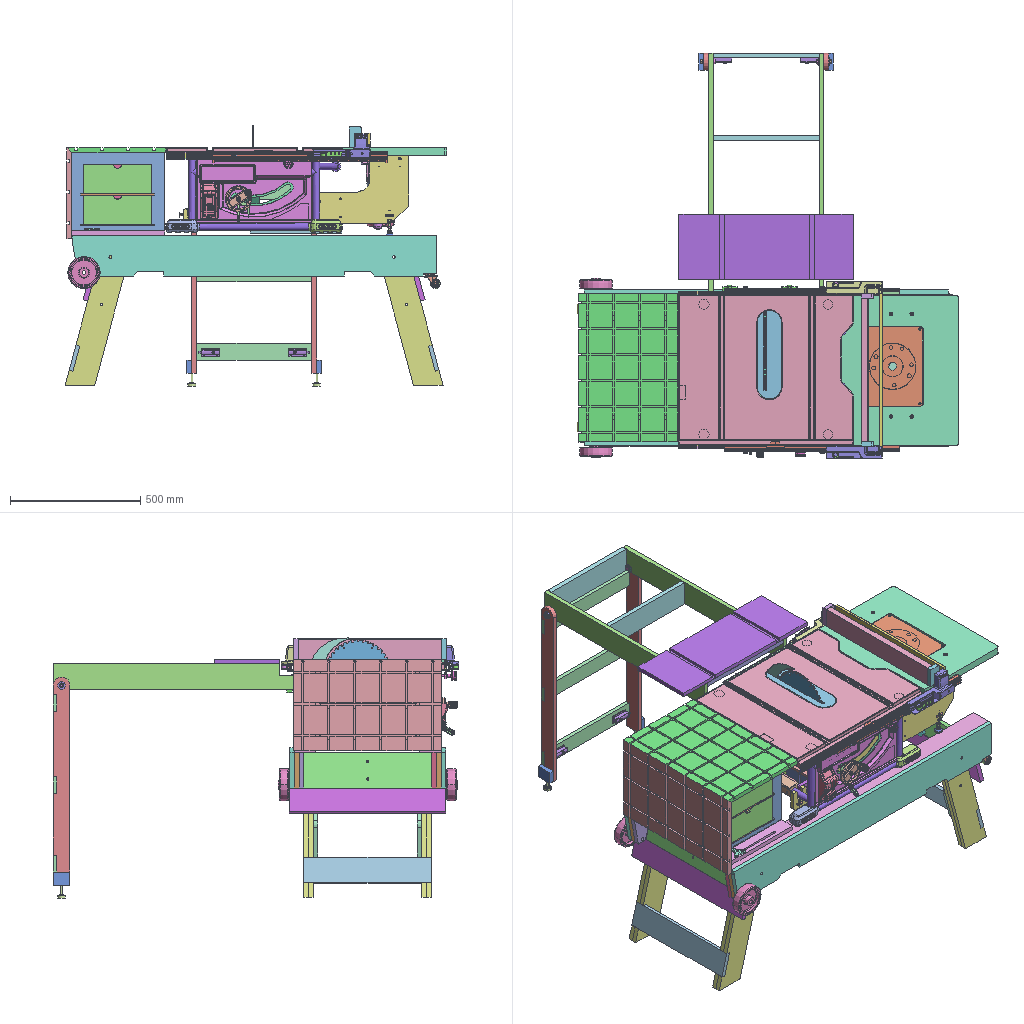Assembly | STEP file | 127 different items | 197 placed | box 1468 x 1560 x 1000 mm
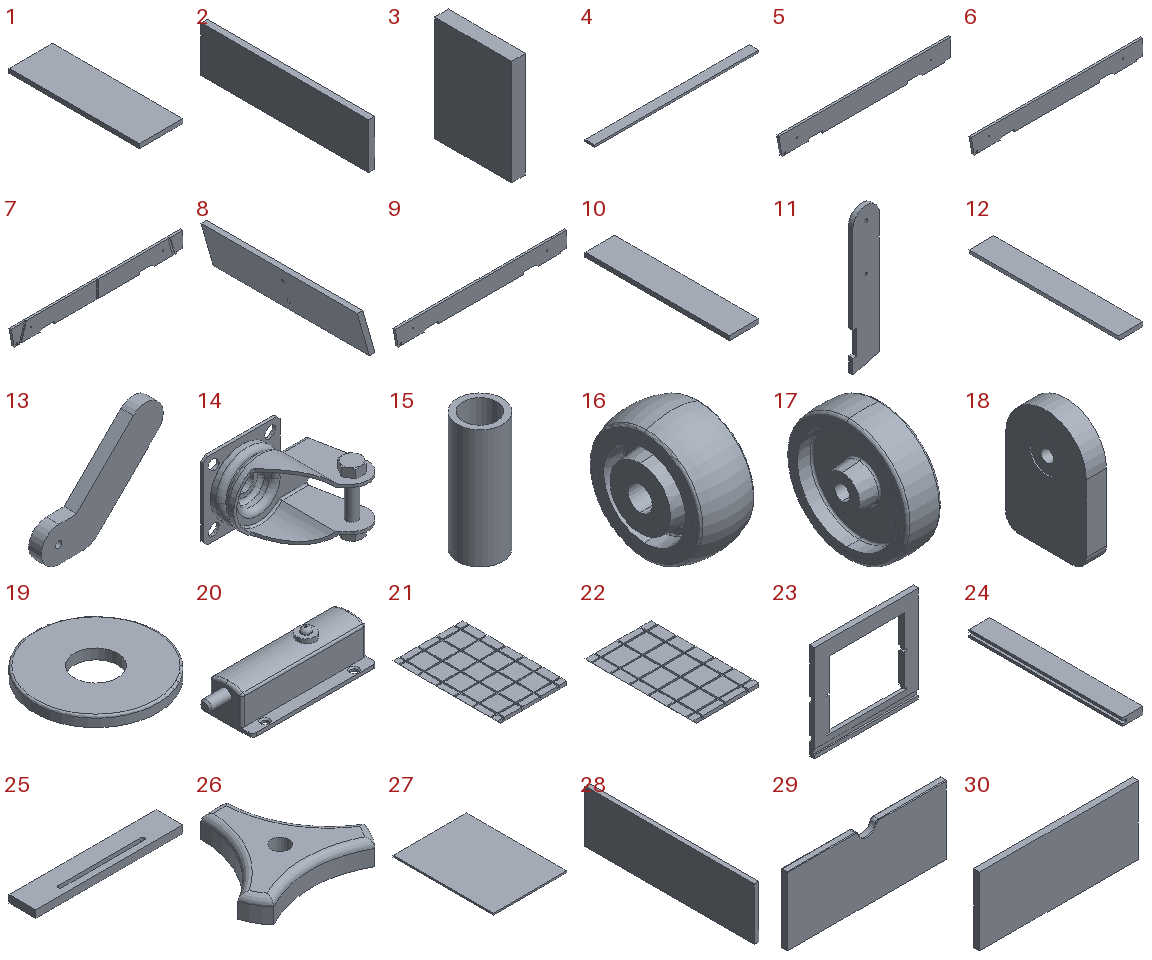Parts list (item | name | quantity | parent item | size | volume):
1 | Frame_top | x1 | in Portable_Workbench_Dwalt7492 | 100 x 300 x 10 mm | 300000 mm3
2 | Middle_part | x1 | in 20 | 18 x 502 x 137 mm | 1237932 mm3
3 | Middle_part | x4 | in 20 | 18 x 100 x 137 mm | 246600 mm3
4 | Frame_right | x2 | in 20 | 1400 x 82 x 18 mm | 2066400 mm3
5 | Frame_right | x2 | in 20 | 1400 x 18 x 155 mm | 3789981 mm3
6 | Frame_right | x2 | in 20 | 1400 x 18 x 137 mm | 3336381 mm3
7 | Frame_right | x1 | in 20 | 1400 x 18 x 137 mm | 3298397 mm3
8 | Frame_top | x2 | in Portable_Workbench_Dwalt7492 | 57.278 x 502 x 136.98 mm | 1235548 mm3
9 | Frame_left | x1 | in 20 | 1400 x 18 x 137 mm | 3298397 mm3
10 | Leg_left | x2 | in 20 | 100 x 490 x 15 mm | 735000 mm3
11 | Leg_left | x8 | in 20 | 110 x 18 x 580.604 mm | 1067190 mm3
12 | Leg_left | x2 | in 20 | 100 x 600 x 18 mm | 1053955 mm3
13 | Leg_right | x2 | in 20 | 174.595 x 18 x 138.64 mm | 178903 mm3
14 | PN_0001 Wheel body | x2 | in 20 | 53 x 48 x 42 mm | 13526 mm3
15 | PN_0001 Wheel body | x2 | in 20 | 8 x 8 x 21 mm | 461.814 mm3
16 | Frame_top | x2 | in Portable_Workbench_Dwalt7492 | 21 x 40 x 40 mm | 18711 mm3
17 | Frame_top | x2 | in Portable_Workbench_Dwalt7492 | 44 x 125 x 125 mm | 224779 mm3
18 | Frame_lock | x2 | in 20 | 15 x 60 x 90 mm | 73219 mm3
19 | Frame_lock | x2 | in 20 | 24 x 24 x 2 mm | 791.374 mm3
20 | Frame_top | x6 | in Portable_Workbench_Dwalt7492, 63 | 82 x 30 x 24.5 mm | 26373 mm3
21 | Superstructure_1 | x1 | in Portable_Workbench_Dwalt7492 | 380 x 570 x 19 mm | 3518605 mm3
22 | Superstructure_1 | x1 | in Portable_Workbench_Dwalt7492 | 350 x 570 x 19 mm | 3268025 mm3
23 | Superstructure_1 | x2 | in Portable_Workbench_Dwalt7492 | 361 x 18 x 336 mm | 1013160 mm3
24 | Superstructure_1 | x4 | in Portable_Workbench_Dwalt7492 | 50 x 374 x 18 mm | 314160 mm3
25 | Superstructure_1 | x2 | in Portable_Workbench_Dwalt7492 | 356.5 x 65 x 18 mm | 383560 mm3
26 | Superstructure_1 | x2 | in Portable_Workbench_Dwalt7492 | 56.861 x 49.792 x 10 mm | 12371 mm3
27 | Drawer | x2 | in 26 | 280 x 382 x 6 mm | 641760 mm3
28 | Drawer | x4 | in 26 | 10 x 362 x 112 mm | 405440 mm3
29 | Drawer | x2 | in 26 | 260 x 10 x 112 mm | 287478 mm3
30 | Drawer | x2 | in 26 | 260 x 10 x 112 mm | 291200 mm3
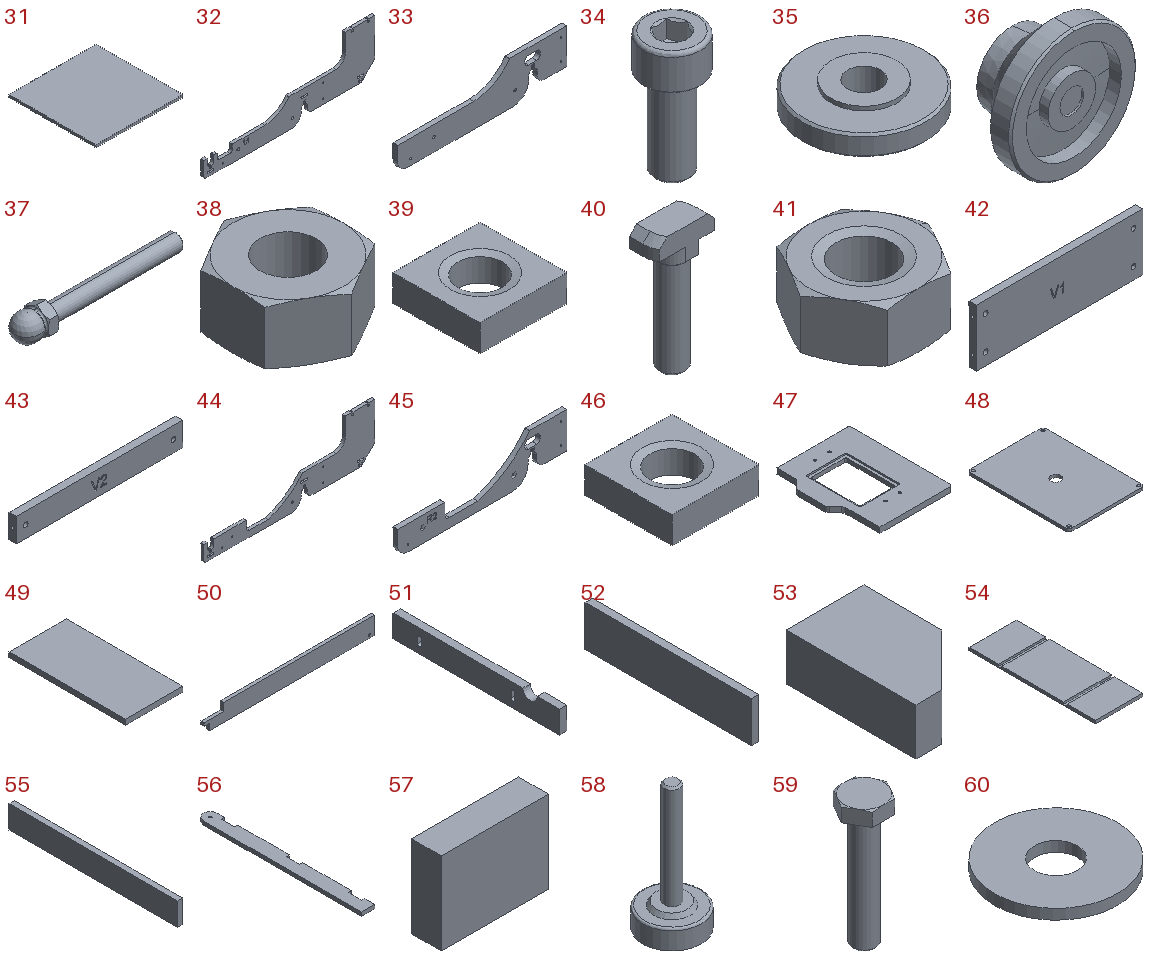31 | Substructure | x1 | in Portable_Workbench_Dwalt7492 | 350 x 350 x 10 mm | 1225000 mm3
32 | Left | x1 | in 48 | 868 x 15 x 287 mm | 1544056 mm3
33 | Left | x1 | in 48 | 575 x 15 x 147 mm | 816987 mm3
34 | Left | x4 | in 48 | 13 x 13 x 28 mm | 1899 mm3
35 | Left | x6 | in 48 | 30 x 30 x 6 mm | 3410 mm3
36 | 343.8-32-M8-63-A | x2 | in 41 | 32 x 15.5 x 32 mm | 6505 mm3
37 | 343.8-32-M8-63-A | x2 | in 41 | 78.67 x 12.5 x 13.856 mm | 4761 mm3
38 | 343.8-32-M8-63-A | x2 | in 41 | 13 x 15.011 x 6.8 mm | 760.328 mm3
39 | Left | x1 | in 48 | 13 x 13 x 4 mm | 530.018 mm3
40 | Left | x4 | in 48 | 18 x 8.32 x 39.5 mm | 2491 mm3
41 | Left | x4 | in 48 | 15.011 x 13 x 6.5 mm | 715.522 mm3
42 | Substructure | x1 | in Portable_Workbench_Dwalt7492 | 350 x 15 x 120 mm | 623484 mm3
43 | Substructure | x1 | in Portable_Workbench_Dwalt7492 | 350 x 15 x 50 mm | 259181 mm3
44 | Right | x1 | in 48 | 866 x 15 x 287 mm | 1373822 mm3
45 | Right | x1 | in 48 | 565 x 15 x 147 mm | 597493 mm3
46 | Right | x1 | in 48 | 13 x 13 x 4 mm | 530.018 mm3
47 | Substructure | x1 | in Portable_Workbench_Dwalt7492 | 453 x 575 x 30 mm | 5515356 mm3
48 | Substructure | x1 | in Portable_Workbench_Dwalt7492 | 228 x 306 x 9 mm | 620161 mm3
49 | Superstructure_3 | x1 | in Portable_Workbench_Dwalt7492 | 200 x 408 x 18 mm | 1468800 mm3
50 | Superstructure_3 | x2 | in Portable_Workbench_Dwalt7492 | 980 x 18 x 100 mm | 1653506 mm3
51 | Superstructure_3 | x1 | in Portable_Workbench_Dwalt7492 | 18 x 408 x 55 mm | 388111 mm3
52 | Superstructure_3 | x2 | in Portable_Workbench_Dwalt7492 | 18 x 408 x 100 mm | 734400 mm3
53 | Superstructure_3 | x2 | in Portable_Workbench_Dwalt7492 | 30 x 50 x 18 mm | 23400 mm3
54 | Superstructure_3 | x1 | in Portable_Workbench_Dwalt7492 | 250 x 670 x 16 mm | 2577227 mm3
55 | Superstructure_3_1 | x3 | in 63 | 15 x 480 x 65 mm | 468000 mm3
56 | Superstructure_3_1 | x2 | in 63 | 65 x 800 x 18 mm | 873479 mm3
57 | Superstructure_3_1 | x2 | in 63 | 65 x 18 x 50 mm | 58500 mm3
58 | Superstructure_3_1 | x2 | in 63 | 30 x 30 x 65 mm | 10178 mm3
59 | Screw_set_M10x45 | x2 | in 63 | 19.63 x 17 x 56.4 mm | 5488 mm3
60 | Screw_set_M10x45 | x2 | in 63 | 30 x 30 x 2.5 mm | 1551 mm3
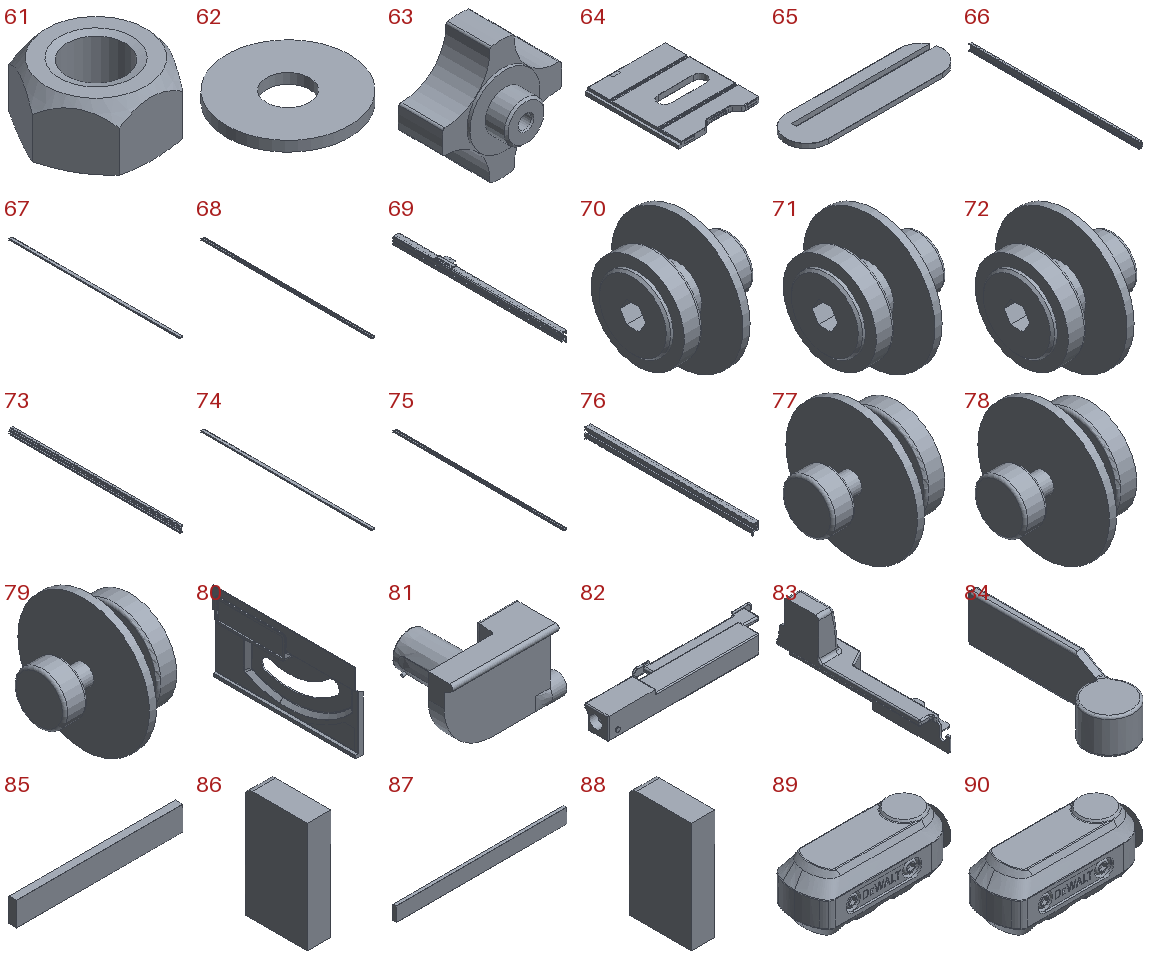61 | Screw_set_M10x45 | x2 | in 63 | 18.475 x 16 x 9 mm | 1440 mm3
62 | Screw_set_M10x45 | x2 | in 63 | 30 x 30 x 2.5 mm | 1551 mm3
63 | Superstructure_3 | x2 | in Portable_Workbench_Dwalt7492 | 60 x 39.998 x 60 mm | 44038 mm3
64 | DEWALT-DWE7492-B22 | x1 | in DeWalt DWE7492 + DWE74911 | 575 x 674 x 40 mm | 781734 mm3
65 | DEWALT-DWE7492-B22 | x1 | in DeWalt DWE7492 + DWE74911 | 342.3 x 93 x 10 mm | 265013 mm3
66 | DEWALT-DWE7492-B22 | x1 | in DeWalt DWE7492 + DWE74911 | 14 x 670 x 25.488 mm | 79850 mm3
67 | DEWALT-DWE7492-B22 | x1 | in DeWalt DWE7492 + DWE74911 | 11.9 x 670 x 4.7 mm | 19402 mm3
68 | DEWALT-DWE7492-B22 | x1 | in DeWalt DWE7492 + DWE74911 | 11.9 x 670 x 4.7 mm | 19402 mm3
69 | DEWALT-DWE7492-B22 | x1 | in DeWalt DWE7492 + DWE74911 | 38.712 x 670 x 45.288 mm | 155212 mm3
70 | DEWALT-DWE7492-B22 | x1 | in DeWalt DWE7492 + DWE74911 | 17.5 x 24 x 24 mm | 1970 mm3
71 | DEWALT-DWE7492-B22 | x1 | in DeWalt DWE7492 + DWE74911 | 17.5 x 24 x 24 mm | 1970 mm3
72 | DEWALT-DWE7492-B22 | x1 | in DeWalt DWE7492 + DWE74911 | 17.5 x 24 x 24 mm | 1970 mm3
73 | DEWALT-DWE7492-B22 | x1 | in DeWalt DWE7492 + DWE74911 | 14 x 670 x 25.488 mm | 79850 mm3
74 | DEWALT-DWE7492-B22 | x1 | in DeWalt DWE7492 + DWE74911 | 11.9 x 670 x 4.7 mm | 19402 mm3
75 | DEWALT-DWE7492-B22 | x1 | in DeWalt DWE7492 + DWE74911 | 11.9 x 670 x 4.7 mm | 19402 mm3
76 | DEWALT-DWE7492-B22 | x1 | in DeWalt DWE7492 + DWE74911 | 24 x 670 x 42.688 mm | 151895 mm3
77 | DEWALT-DWE7492-B22 | x1 | in DeWalt DWE7492 + DWE74911 | 17.5 x 24 x 24 mm | 1970 mm3
78 | DEWALT-DWE7492-B22 | x1 | in DeWalt DWE7492 + DWE74911 | 17.5 x 24 x 24 mm | 1970 mm3
79 | DEWALT-DWE7492-B22 | x1 | in DeWalt DWE7492 + DWE74911 | 17.5 x 24 x 24 mm | 1970 mm3
80 | DEWALT-DWE7492-B22 | x1 | in DeWalt DWE7492 + DWE74911 | 29 x 440 x 245 mm | 127780 mm3
81 | DEWALT-DWE7492-B2_23 | x1 | in 102 | 375 x 265.806 x 237.3 mm | 6943918 mm3
82 | DEWALT-DWE7492-B22 | x1 | in DeWalt DWE7492 + DWE74911 | 365.575 x 76.384 x 45 mm | 432829 mm3
83 | DEWALT-DWE7492-B2_002 | x1 | in 102 | 48.75 x 241 x 100.5 mm | 225143 mm3
84 | DEWALT-DWE7492-B2_002 | x1 | in 102 | 21.679 x 79.466 x 21.2 mm | 10933 mm3
85 | DEWALT-DWE7492-B22 | x1 | in DeWalt DWE7492 + DWE74911 | 552.2 x 25.6 x 80 mm | 1130787 mm3
86 | DEWALT-DWE7492-B22 | x1 | in DeWalt DWE7492 + DWE74911 | 17 x 45 x 80 mm | 61109 mm3
87 | DEWALT-DWE7492-B22 | x1 | in DeWalt DWE7492 + DWE74911 | 586.2 x 11 x 50 mm | 322284 mm3
88 | DEWALT-DWE7492-B22 | x1 | in DeWalt DWE7492 + DWE74911 | 17 x 45 x 80 mm | 61109 mm3
89 | DEWALT-DWE7492-B22 | x1 | in DeWalt DWE7492 + DWE74911 | 128.5 x 51.395 x 52 mm | 252814 mm3
90 | DEWALT-DWE7492-B22 | x1 | in DeWalt DWE7492 + DWE74911 | 128.5 x 51.395 x 52 mm | 252814 mm3
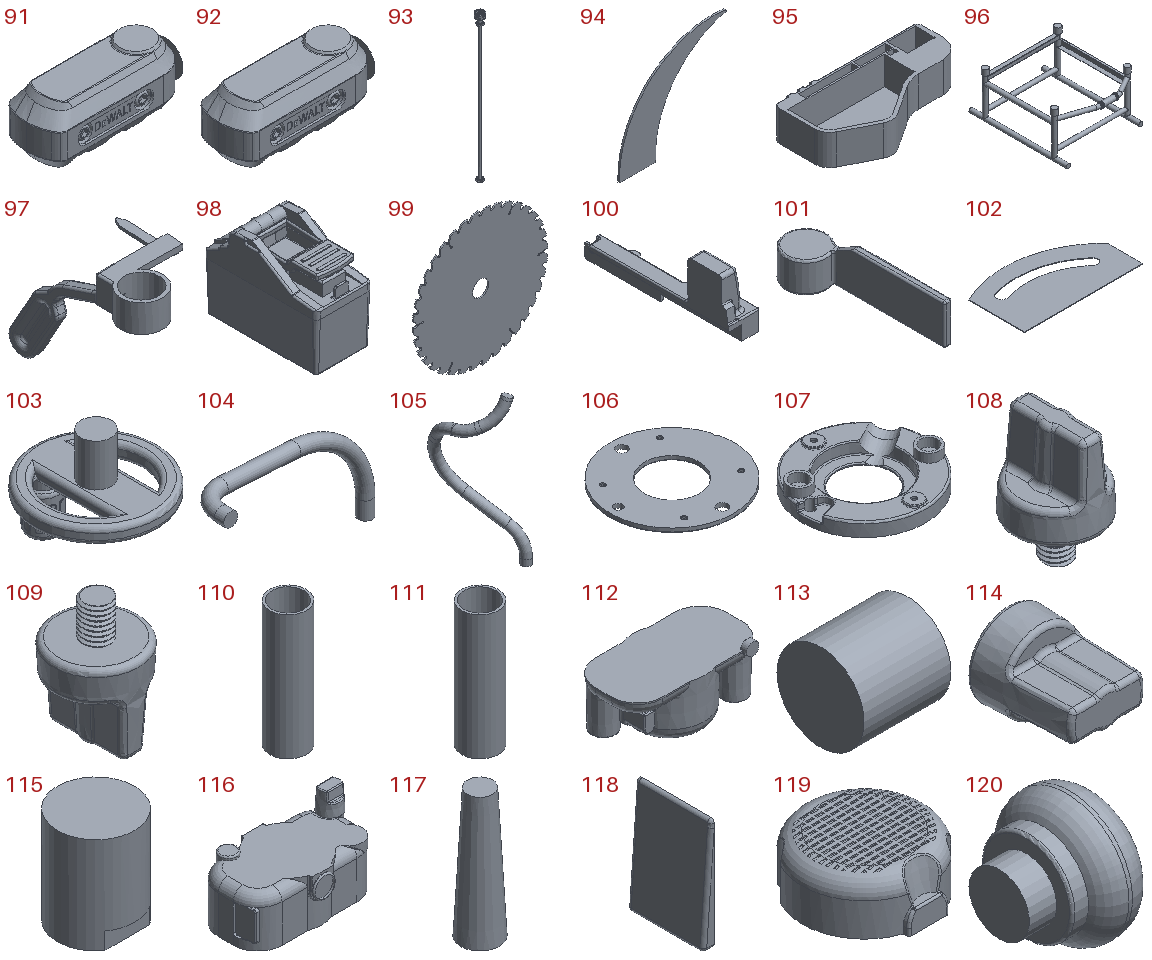91 | DEWALT-DWE7492-B22 | x1 | in DeWalt DWE7492 + DWE74911 | 128.5 x 51.395 x 52 mm | 252814 mm3
92 | DEWALT-DWE7492-B22 | x1 | in DeWalt DWE7492 + DWE74911 | 128.5 x 51.395 x 52 mm | 252814 mm3
93 | DEWALT-DWE7294-B2-35 | x1 | in 102 | 36.143 x 35.85 x 635.164 mm | 52230 mm3
94 | DEWALT-DWE7492-B22 | x1 | in DeWalt DWE7492 + DWE74911 | 159.2 x 2.5 x 146.092 mm | 19224 mm3
95 | DEWALT-DWE7492-B22 | x1 | in DeWalt DWE7492 + DWE74911 | 126.934 x 64.887 x 27 mm | 57181 mm3
96 | DEWALT-DWE7492-B22 | x1 | in DeWalt DWE7492 + DWE74911 | 540.27 x 670 x 316.25 mm | 3162222 mm3
97 | DEWALT-DWE7492-B22 | x1 | in DeWalt DWE7492 + DWE74911 | 57.196 x 108.227 x 84.374 mm | 18849 mm3
98 | DEWALT-DWE7492-B22 | x1 | in DeWalt DWE7492 + DWE74911 | 68 x 135 x 106.953 mm | 732331 mm3
99 | DEWALT-DWE7492-B22 | x1 | in DeWalt DWE7492 + DWE74911 | 249.95 x 2.5 x 249.95 mm | 115629 mm3
100 | DEWALT-DWE7492-B2_25_zrc002 | x1 | in 102 | 48.75 x 241 x 100.5 mm | 225143 mm3
101 | DEWALT-DWE7492-B2_25_zrc002 | x1 | in 102 | 21.679 x 79.466 x 21.2 mm | 10933 mm3
102 | DEWALT-DWE7492-B22 | x1 | in DeWalt DWE7492 + DWE74911 | 310 x 173.249 x 1.5 mm | 62971 mm3
103 | DEWALT-DWE7294-B3-01 | x1 | in 102 | 102 x 108.2 x 94.708 mm | 107862 mm3
104 | DEWALT-DWE7294-B3-02 | x1 | in 102 | 105.161 x 24.081 x 60.688 mm | 7333 mm3
105 | DEWALT-DWE7294-B3-03 | x1 | in 102 | 51.027 x 77.706 x 165.503 mm | 18773 mm3
106 | Slide_plate | x1 | in 127 | 180 x 180 x 6 mm | 116281 mm3
107 | Base_plate_001 | x1 | in 127 | 180 x 180 x 32.5 mm | 306829 mm3
108 | Base_plate_001 | x1 | in 127 | 23.839 x 23.839 x 34 mm | 6540 mm3
109 | Base_plate_001 | x1 | in 127 | 23.839 x 23.839 x 34 mm | 6540 mm3
110 | CMT7E v7 | x1 | in Portable_Workbench_Dwalt7492 | 25 x 25 x 85 mm | 9413 mm3
111 | CMT7E v7 | x1 | in Portable_Workbench_Dwalt7492 | 25 x 25 x 85 mm | 9413 mm3
112 | Lower_shell_0 | x1 | in 114 | 190 x 106.5 x 113 mm | 927273 mm3
113 | Lower_shell_0 | x1 | in 114 | 10 x 10 x 10 mm | 785.398 mm3
114 | Lower_shell | x1 | in 127 | 26.929 x 33 x 26.929 mm | 11981 mm3
115 | CMT7E v7 | x1 | in Portable_Workbench_Dwalt7492 | 32 x 32 x 40 mm | 31637 mm3
116 | Upper_shell_sub | x1 | in 127 | 200.312 x 115 x 105 mm | 1313356 mm3
117 | Upper_shell_sub | x1 | in 127 | 15 x 15 x 50 mm | 6108 mm3
118 | Upper_shell_sub | x1 | in 127 | 3.182 x 22 x 32.446 mm | 1438 mm3
119 | CMT7E v7 | x1 | in Portable_Workbench_Dwalt7492 | 105 x 109 x 43 mm | 352834 mm3
120 | CMT7E v7 | x1 | in Portable_Workbench_Dwalt7492 | 53 x 68 x 68 mm | 121265 mm3
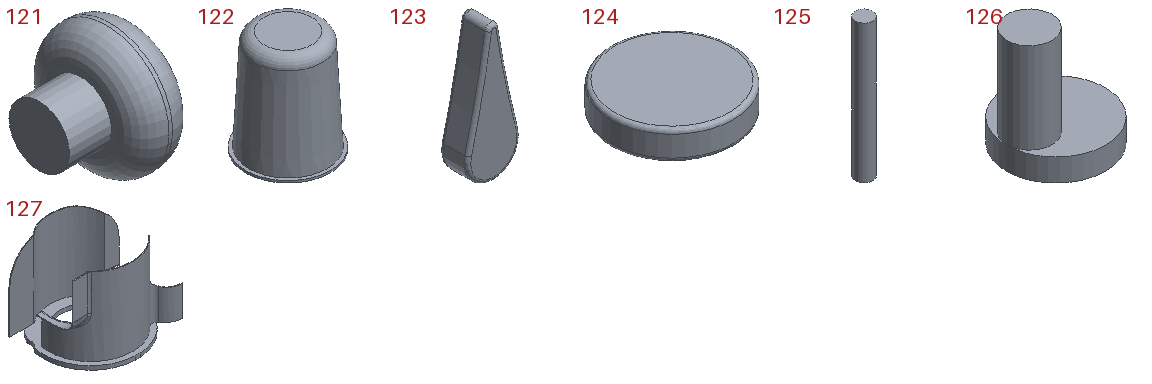121 | CMT7E v7 | x1 | in Portable_Workbench_Dwalt7492 | 53 x 68 x 68 mm | 112304 mm3
122 | CMT7E v7 | x1 | in Portable_Workbench_Dwalt7492 | 40 x 40 x 48 mm | 44913 mm3
123 | CMT7E v7 | x1 | in Portable_Workbench_Dwalt7492 | 23 x 12 x 59 mm | 9832 mm3
124 | CMT7E v7 | x1 | in Portable_Workbench_Dwalt7492 | 29.77 x 29.77 x 7 mm | 4833 mm3
125 | CMT7E v7 | x1 | in Portable_Workbench_Dwalt7492 | 10 x 10 x 80 mm | 6283 mm3
126 | CMT7E v7 | x1 | in Portable_Workbench_Dwalt7492 | 22 x 22 x 25 mm | 3472 mm3
127 | CMT7E v7 | x1 | in Portable_Workbench_Dwalt7492 | 132.537 x 120.91 x 105 mm | 56279 mm3
Placements (level | parent | child | x y z in mm | rotation matrix by rows):
1 | Portable_Workbench_Dwalt7492 | Portable_Workbench_Dwalt7492 | 0.0 0.0 0.0 | 1 0 0 0 1 0 0 0 1
2 | Portable_Workbench_Dwalt7492 | Frame_top | 0.0 0.0 0.0 | 1 0 0 0 1 0 0 0 1
2 | Portable_Workbench_Dwalt7492 | Frame_top | 0.0 0.0 -86.5 | 1 0 0 0 1 0 0 0 1
3 | Frame_top | Middle_part | 0.0 0.0 0.0 | 1 0 0 0 1 0 0 0 1
3 | Frame_top | Middle_part | 9.0 158.0 0.0 | 1 0 0 0 1 0 0 0 1
3 | Frame_top | Middle_part | 9.0 -158.0 0.0 | 1 0 0 0 1 0 0 0 1
3 | Frame_top | Middle_part | -27.0 158.0 0.0 | 1 0 0 0 1 0 0 0 1
3 | Frame_top | Middle_part | -27.0 -158.0 0.0 | 1 0 0 0 1 0 0 0 1
2 | Portable_Workbench_Dwalt7492 | Frame_top | 0.0 241.0 -18.0 | 1 0 0 0 1 0 0 0 1
3 | Frame_top | Frame_right | 0.0 0.0 0.0 | 1 0 0 0 1 0 0 0 1
3 | Frame_top | Frame_right | 0.0 59.0 -59.5 | 1 0 0 0 1 0 0 0 1
3 | Frame_top | Frame_right | 0.0 41.0 -68.5 | 1 0 0 0 1 0 0 0 1
3 | Frame_top | Frame_right | 0.0 23.0 -68.5 | 1 0 0 0 1 0 0 0 1
2 | Portable_Workbench_Dwalt7492 | Frame_top | 606.426 0.0 -89.27 | 1 0 0 0 1 0 0 0 1
2 | Portable_Workbench_Dwalt7492 | Frame_top | -606.269 -0.0 -89.27 | -1 0 0 0 -1 0 0 0 1
2 | Portable_Workbench_Dwalt7492 | Frame_top | 0.0 -241.0 -18.0 | 1 0 0 0 1 0 0 0 1
3 | Frame_top | Frame_right | 0.0 0.0 0.0 | 1 0 0 0 1 0 0 0 1
3 | Frame_top | Frame_right | -0.0 -41.0 -59.5 | 1 0 0 0 1 0 0 0 1
3 | Frame_top | Frame_left | 0.0 -5.0 -68.5 | 1 0 0 0 1 0 0 0 1
3 | Frame_top | Frame_right | 0.0 -23.0 -68.5 | 1 0 0 0 1 0 0 0 1
2 | Portable_Workbench_Dwalt7492 | Frame_top | -690.847 1.0 -471.145 | 0.2588 0 -0.9659 0 1 0 0.9659 0 0.2588
3 | Frame_top | Leg_left | 0.0 0.0 0.0 | 1 0 0 0 1 0 0 0 1
3 | Frame_top | Leg_left | 415.6 -209.0 -47.5 | 0 0 1 0 1 0 -1 0 -0
3 | Frame_top | Leg_left | 415.6 -227.0 -47.5 | 0 0 1 0 1 0 -1 0 -0
3 | Frame_top | Leg_left | 415.6 245.0 -47.5 | 0 0 1 0 1 0 -1 0 -0
3 | Frame_top | Leg_left | 415.6 227.0 -47.5 | 0 0 1 0 1 0 -1 0 -0
3 | Frame_top | Leg_left | 275.0 -0.0 16.5 | -1 0 0 0 1 0 0 0 -1
2 | Portable_Workbench_Dwalt7492 | Frame_top | 690.648 1.0 -471.149 | -0.2588 0 0.9659 0 -1 0 0.9659 0 0.2588
3 | Frame_top | Leg_left | 0.0 0.0 0.0 | 1 0 0 0 1 0 0 0 1
3 | Frame_top | Leg_left | 415.604 -209.0 -47.5 | 0 0 1 0 1 0 -1 0 0
3 | Frame_top | Leg_left | 415.604 -227.0 -47.5 | 0 0 1 0 1 0 -1 0 -0
3 | Frame_top | Leg_left | 415.604 245.0 -47.5 | 0 0 1 0 1 0 -1 0 0
3 | Frame_top | Leg_left | 415.604 227.0 -47.5 | 0 0 1 0 1 0 -1 0 -0
3 | Frame_top | Leg_left | 275.0 -0.0 16.5 | -1 0 0 0 1 0 0 0 -1
3 | Frame_top | Leg_right | 225.604 191.0 -47.5 | -0.7108 0 -0.7034 0 -1 0 -0.7034 0 0.7108
3 | Frame_top | Leg_right | 225.604 -209.0 -47.5 | -0.7108 0 -0.7034 0 -1 0 -0.7034 0 0.7108
2 | Portable_Workbench_Dwalt7492 | Frame_top | 674.0 273.0 -146.5 | 1 0 0 0 0 -1 0 1 -0
3 | Frame_top | PN_0001 Wheel body | 0.0 0.0 0.0 | 1 0 0 0 1 0 0 0 1
3 | Frame_top | PN_0001 Wheel body | 0.0 0.0 0.0 | 1 0 0 0 1 0 0 0 1
2 | Portable_Workbench_Dwalt7492 | Frame_top | 674.0 -273.0 -146.5 | 1 0 0 0 0 -1 0 1 -0
3 | Frame_top | PN_0001 Wheel body | 0.0 0.0 0.0 | 1 0 0 0 1 0 0 0 1
3 | Frame_top | PN_0001 Wheel body | 0.0 0.0 0.0 | 1 0 0 0 1 0 0 0 1
2 | Portable_Workbench_Dwalt7492 | Frame_top | 697.0 273.0 -184.0 | 0 1 0 -1 0 0 0 0 1
2 | Portable_Workbench_Dwalt7492 | Frame_top | 697.0 -273.0 -184.0 | 0 1 0 -1 0 0 0 0 1
2 | Portable_Workbench_Dwalt7492 | Frame_top | -653.843 -322.0 -142.0 | 0 0 -1 -1 0 0 0 1 0
2 | Portable_Workbench_Dwalt7492 | Frame_top | -653.843 322.0 -142.0 | 0 0 -1 1 0 0 0 -1 0
2 | Portable_Workbench_Dwalt7492 | Frame_top | -606.64 -0.0 -125.575 | 0.9613 -0.2756 0.001192 0 0.004323 1 -0.2756 -0.9613 0.004156
3 | Frame_top | Frame_lock | 0.0 0.0 0.0 | 1 0 0 0 1 0 0 0 1
3 | Frame_top | Frame_lock | 1.0 0.0 0.0 | 0 0 -1 1 0 0 0 -1 0
2 | Portable_Workbench_Dwalt7492 | Frame_top | 606.797 0.0 -125.575 | -0.9613 0.2756 0 0 0 -1 -0.2756 -0.9613 0
3 | Frame_top | Frame_lock | 0.0 0.0 0.0 | 1 0 0 0 1 0 0 0 1
3 | Frame_top | Frame_lock | 1.0 0.0 0.0 | 0 0 -1 1 0 0 0 -1 0
2 | Portable_Workbench_Dwalt7492 | Frame_top | -27.0 204.0 -115.0 | 0 0 -1 -1 0 0 0 1 -0
2 | Portable_Workbench_Dwalt7492 | Frame_top | -27.0 -204.0 -115.0 | 0 0 -1 1 0 0 0 -1 -0
2 | Portable_Workbench_Dwalt7492 | Frame_top | 27.0 204.0 -115.0 | 0 0 1 -1 0 0 0 -1 0
2 | Portable_Workbench_Dwalt7492 | Frame_top | 27.0 -204.0 -115.0 | 0 0 1 1 0 0 0 1 0
1 | Portable_Workbench_Dwalt7492 | Portable_Workbench_Dwalt7492 | -530.0 -0.0 328.5 | 1 0 0 0 1 0 0 0 1
2 | Portable_Workbench_Dwalt7492 | Superstructure_1 | 0.0 0.0 0.0 | 1 0 0 0 1 0 0 0 1
2 | Portable_Workbench_Dwalt7492 | Superstructure_1 | -180.5 0.0001 -165.5 | 0 0 -1 0 -1 0 -1 0 0
2 | Portable_Workbench_Dwalt7492 | Superstructure_1 | 5 -191.0 -172.5 | 1 0 0 0 1 0 0 0 1
2 | Portable_Workbench_Dwalt7492 | Superstructure_1 | 5 191.0 -172.5 | -1 0 0 0 -1 0 0 0 1
2 | Portable_Workbench_Dwalt7492 | Superstructure_1 | -151.0 0.0 -169.5 | -1 0 0 0 -1 0 0 0 1
2 | Portable_Workbench_Dwalt7492 | Superstructure_1 | -151.0 0.0 -287.5 | -1 0 0 0 -1 0 0 0 1
2 | Portable_Workbench_Dwalt7492 | Superstructure_1 | 160.5 -0.0001 -169.5 | 1 0 0 0 1 0 0 0 1
2 | Portable_Workbench_Dwalt7492 | Superstructure_1 | 160.5 -0.0001 -287.5 | 1 0 0 0 1 0 0 0 1
2 | Portable_Workbench_Dwalt7492 | Superstructure_1 | 7.5 -227.5 -319.5 | 1 0 0 0 1 0 0 0 1
2 | Portable_Workbench_Dwalt7492 | Superstructure_1 | 7.5 227.5 -319.5 | -1 0 0 0 -1 0 0 0 1
2 | Portable_Workbench_Dwalt7492 | Superstructure_1 | -92.5 -240.5 -310.5 | -0.4805 -0.877 0 0.877 -0.4805 0 0 0 1
2 | Portable_Workbench_Dwalt7492 | Superstructure_1 | -92.5 240.5 -310.5 | 0.4984 0.867 0 -0.867 0.4984 0 0 0 1
2 | Portable_Workbench_Dwalt7492 | Superstructure_1 | 5.0 -10.0 -290.5 | 1 0 0 0 1 0 0 0 1
3 | Superstructure_1 | Drawer | 0.0 0.0 0.0 | 1 0 0 0 1 0 0 0 1
3 | Superstructure_1 | Drawer | -125.0 -0.0 6.0 | 1 0 0 0 1 0 0 0 1
3 | Superstructure_1 | Drawer | 125.0 0.0 6.0 | 1 0 0 0 1 0 0 0 1
3 | Superstructure_1 | Drawer | 0.0 -181.0 6.0 | 1 0 0 0 1 0 0 0 1
3 | Superstructure_1 | Drawer | 0.0 191.0 6.0 | 1 0 0 0 1 0 0 0 1
2 | Portable_Workbench_Dwalt7492 | Superstructure_1 | 5.0 -10.0 -172.5 | 1 0 0 0 1 0 0 0 1
3 | Superstructure_1 | Drawer | 0.0 0.0 0.0 | 1 0 0 0 1 0 0 0 1
3 | Superstructure_1 | Drawer | -125.0 -0.0 6.0 | 1 0 0 0 1 0 0 0 1
3 | Superstructure_1 | Drawer | 125.0 0.0 6.0 | 1 0 0 0 1 0 0 0 1
3 | Superstructure_1 | Drawer | 0.0 -181.0 6.0 | 1 0 0 0 1 0 0 0 1
3 | Superstructure_1 | Drawer | 0.0 191.0 6.0 | 1 0 0 0 1 0 0 0 1
1 | Portable_Workbench_Dwalt7492 | Portable_Workbench_Dwalt7492 | 161.0 9.5 20.0 | 1 0 0 0 1 0 0 0 1
2 | Portable_Workbench_Dwalt7492 | Substructure | 0.0 0.0 0.0 | 1 0 0 0 1 0 0 0 1
2 | Portable_Workbench_Dwalt7492 | Substructure | 434.0 -190.0 0.0 | 1 0 0 0 1 0 0 0 1
3 | Substructure | Left | 0.0 0.0 0.0 | 1 0 0 0 1 0 0 0 1
3 | Substructure | Left | 0.0 15.0 0.0 | 1 0 0 0 1 0 0 0 1
3 | Substructure | Left | -419.0 -6.0 45.0 | -1 0 0 0 0 -1 0 -1 0
3 | Substructure | Left | -694.0 -6.0 45.0 | -1 0 0 0 0 -1 0 -1 0
3 | Substructure | Left | -74.0 -7.5 59.0 | 1 0 0 0 -1 0 0 0 -1
3 | Substructure | Left | -74.0 -7.5 -23.17 | 0 0 1 1 0 0 0 1 0
4 | Left | 343.8-32-M8-63-A | 0.0 0.0 0.0 | 1 0 0 0 1 0 0 0 1
4 | Left | 343.8-32-M8-63-A | 0.0 22.67 0.0 | 0 -1 0 1 0 0 0 0 1
4 | Left | 343.8-32-M8-63-A | 0.0 36.07 0.0 | 0.5 -0.866 0 0 0 1 -0.866 -0.5 0
3 | Substructure | Left | -74.0 -7.5 32.0 | -1 0 0 0 -1 0 0 0 1
3 | Substructure | Left | -834.0 -7.5 17.5 | 1 0 0 0 1 0 0 0 1
3 | Substructure | Left | -358.5 -7.5 113.0 | -1 0 0 0 1 0 0 0 -1
3 | Substructure | Left | -834.0 -7.5 32.16 | 0 1 0 -1 0 0 0 0 1
3 | Substructure | Left | -694.0 13.5 45.0 | -1 0 0 0 0 -1 0 -1 -0
3 | Substructure | Left | -419.0 13.5 45.0 | -1 0 0 0 0 -1 0 -1 -0
3 | Substructure | Left | -358.5 -7.5 85.84 | 0 -1 0 -1 0 0 0 0 -1
2 | Portable_Workbench_Dwalt7492 | Substructure | 178.5 0.0 87.0 | 0 1 0 -1 0 0 0 0 1
2 | Portable_Workbench_Dwalt7492 | Substructure | -339.0 0.0 22.0 | 0 0 -1 1 0 0 0 -1 0
2 | Portable_Workbench_Dwalt7492 | Substructure | 434.0 205.0 0.0 | 1 0 0 0 1 0 0 0 1
3 | Substructure | Right | 0.0 0.0 0.0 | 1 0 0 0 1 0 0 0 1
3 | Substructure | Right | 0.0 -15.0 0.0 | 1 0 0 0 1 0 0 0 1
3 | Substructure | Right | -74.0 -7.5 32.5 | -1 0 0 0 -1 0 0 0 1
3 | Substructure | Left | -74.0 -7.5 59.0 | -1 0 0 0 1 0 0 0 -1
3 | Substructure | Left | -74.0 -7.5 -23.17 | 0 0 1 1 0 0 0 1 -0
4 | Left | 343.8-32-M8-63-A | 0.0 0.0 0.0 | 1 0 0 0 1 0 0 0 1
4 | Left | 343.8-32-M8-63-A | 0.0 22.67 0.0 | 0 -1 0 1 0 0 0 0 1
4 | Left | 343.8-32-M8-63-A | 0.0 36.07 0.0 | 0.5 -0.866 0 0 0 1 -0.866 -0.5 0
3 | Substructure | Left | -358.5 -7.5 113.0 | 1 0 0 0 -1 0 0 0 -1
3 | Substructure | Left | -358.5 -7.5 85.84 | 0 1 0 1 0 0 0 0 -1
3 | Substructure | Left | -832.0 -7.5 17.5 | 1 0 0 0 1 0 0 0 1
3 | Substructure | Left | -832.0 -7.5 31.16 | 0 -1 0 1 0 0 0 0 1
3 | Substructure | Left | -419.0 -9.335 45.0 | 1 0 0 0 0 1 0 -1 -0
3 | Substructure | Left | -724.0 -9.0 45.0 | 1 0 0 0 0 1 0 -1 -0
3 | Substructure | Left | -419.0 -28.5 45.0 | -1 0 0 0 0 1 0 1 0
3 | Substructure | Left | -724.0 -28.5 45.0 | -1 0 0 0 0 1 0 1 0
2 | Portable_Workbench_Dwalt7492 | Substructure | 327.5 -20.0 318.0 | 1 0 0 0 1 0 0 0 1
2 | Portable_Workbench_Dwalt7492 | Substructure | 325.0 -4 315.0 | 1 0 0 0 1 0 0 0 1
1 | Portable_Workbench_Dwalt7492 | Portable_Workbench_Dwalt7492 | 0.0 439.5 322.0 | 0 -1 0 1 0 0 0 0 1
2 | Portable_Workbench_Dwalt7492 | Superstructure_3 | 0.0 0.0 -9.0 | 1 0 0 0 1 0 0 0 1
2 | Portable_Workbench_Dwalt7492 | Superstructure_3 | -180.0 -213.0 -100.0 | 1 0 0 0 1 0 0 0 1
2 | Portable_Workbench_Dwalt7492 | Superstructure_3 | -180.0 213.0 -100.0 | 1 0 0 0 1 0 0 0 1
2 | Portable_Workbench_Dwalt7492 | Superstructure_3 | -171.0 -0.0 -72.5 | 1 0 0 0 1 0 0 0 1
2 | Portable_Workbench_Dwalt7492 | Superstructure_3 | 761.0 0.0 -50.0 | 1 0 0 0 1 0 0 0 1
2 | Portable_Workbench_Dwalt7492 | Superstructure_3 | 443.0 0.0 -50.0 | 1 0 0 0 1 0 0 0 1
2 | Portable_Workbench_Dwalt7492 | Superstructure_3 | -195.0 -179.0 -54.0 | -1 0 0 0 -1 0 0 0 1
2 | Portable_Workbench_Dwalt7492 | Superstructure_3 | -195.0 179.0 -54.0 | -1 0 0 0 1 0 0 0 -1
2 | Portable_Workbench_Dwalt7492 | Superstructure_3 | 25.0 0.0 16.0 | 1 0 0 0 1 0 0 0 1
2 | Portable_Workbench_Dwalt7492 | Superstructure_3 | 737.5 -0.0 -82.5 | 1 0 0 0 1 0 0 0 1
3 | Superstructure_3 | Superstructure_3_1 | 25.0 0.0 -67.5 | 1 0 0 0 1 0 0 0 1
3 | Superstructure_3 | Superstructure_3_1 | -0.0 -231.0 0.0 | 1 0 0 0 0 -1 0 1 -0
3 | Superstructure_3 | Superstructure_3_1 | 0.0 231.0 -0.0 | 1 0 0 0 0 -1 0 1 -0
3 | Superstructure_3 | Superstructure_3_1 | 25.0 0.0 -383.75 | 1 0 0 0 1 0 0 0 1
3 | Superstructure_3 | Superstructure_3_1 | 25.0 0.0 -685.0 | 1 0 0 0 1 0 0 0 1
3 | Superstructure_3 | Superstructure_3_1 | 0.0 -249.0 -767.5 | 1 0 0 0 1 0 0 0 1
3 | Superstructure_3 | Superstructure_3_1 | -0.0 249.0 -767.5 | 1 0 0 0 1 0 0 0 1
3 | Superstructure_3 | Frame_top | 17.5 -202.0 -687.5 | 0 0 -1 1 0 0 0 -1 -0
3 | Superstructure_3 | Frame_top | 17.5 202.0 -687.5 | 0 0 -1 -1 0 0 0 1 0
3 | Superstructure_3 | Superstructure_3_1 | -0.0 240.0 -817.5 | 1 0 0 0 1 0 0 0 1
3 | Superstructure_3 | Superstructure_3_1 | 0.0 -240.0 -817.5 | 1 0 0 0 1 0 0 0 1
2 | Portable_Workbench_Dwalt7492 | Superstructure_3 | 737.5 -201.5 -82.5 | 1 0 0 0 0 1 0 -1 0
3 | Superstructure_3 | Screw_set_M10x45 | 0.0 0.0 0.0 | 1 0 0 0 1 0 0 0 1
3 | Superstructure_3 | Screw_set_M10x45 | 0.0 0.0 -2.5 | 1 0 0 0 1 0 0 0 1
3 | Superstructure_3 | Screw_set_M10x45 | 0.0 0.0 -41.0 | 1 0 0 0 -1 0 0 0 -1
3 | Superstructure_3 | Screw_set_M10x45 | 0.0 0.0 -41.0 | 1 0 0 0 1 0 0 0 1
2 | Portable_Workbench_Dwalt7492 | Superstructure_3 | 737.5 201.5 -82.5 | 0 -1 0 0 0 -1 1 0 0
3 | Superstructure_3 | Screw_set_M10x45 | 0.0 0.0 0.0 | 1 0 0 0 1 0 0 0 1
3 | Superstructure_3 | Screw_set_M10x45 | 0.0 0.0 -2.5 | 1 0 0 0 1 0 0 0 1
3 | Superstructure_3 | Screw_set_M10x45 | 0.0 0.0 -41.0 | 1 0 0 0 -1 0 0 0 -1
3 | Superstructure_3 | Screw_set_M10x45 | 0.0 0.0 -41.0 | 1 0 0 0 1 0 0 0 1
2 | Portable_Workbench_Dwalt7492 | Superstructure_3 | -150.0 -90.0 -80.0 | 0 1 0 0 0 -1 -1 0 0
2 | Portable_Workbench_Dwalt7492 | Superstructure_3 | -150.0 139.5 -80.0 | 0 1 0 0 0 -1 -1 0 0
1 | Portable_Workbench_Dwalt7492 | Portable_Workbench_Dwalt7492 | -0.0 -0.0 298.0 | 0 -1 0 1 0 0 0 0 1
2 | Portable_Workbench_Dwalt7492 | DeWalt DWE7492 + DWE74911 | 0.0 0.0 0.0 | 1 0 0 0 1 0 0 0 1
3 | DeWalt DWE7492 + DWE74911 | DEWALT-DWE7492-B22 | 0.0 0.0 0.0 | 1 0 0 0 1 0 0 0 1
3 | DeWalt DWE7492 + DWE74911 | DEWALT-DWE7492-B22 | 0.0 0.0 0.0 | 1 0 0 0 1 0 0 0 1
3 | DeWalt DWE7492 + DWE74911 | DEWALT-DWE7492-B22 | 0.0 0.0 0.0 | 1 0 0 0 1 0 0 0 1
3 | DeWalt DWE7492 + DWE74911 | DEWALT-DWE7492-B22 | 0.0 0.0 0.0 | 1 0 0 0 1 0 0 0 1
3 | DeWalt DWE7492 + DWE74911 | DEWALT-DWE7492-B22 | 0.0 0.0 0.0 | 1 0 0 0 1 0 0 0 1
3 | DeWalt DWE7492 + DWE74911 | DEWALT-DWE7492-B22 | 0.0 -176.122 0.0 | 1 0 0 0 1 0 0 0 1
3 | DeWalt DWE7492 + DWE74911 | DEWALT-DWE7492-B22 | 0.0 -176.122 0.0 | 1 0 0 0 1 0 0 0 1
3 | DeWalt DWE7492 + DWE74911 | DEWALT-DWE7492-B22 | 0.0 -176.122 0.0 | 1 0 0 0 1 0 0 0 1
3 | DeWalt DWE7492 + DWE74911 | DEWALT-DWE7492-B22 | 0.0 -176.122 0.0 | 1 0 0 0 1 0 0 0 1
3 | DeWalt DWE7492 + DWE74911 | DEWALT-DWE7492-B22 | 0.0 0.0 0.0 | 1 0 0 0 1 0 0 0 1
3 | DeWalt DWE7492 + DWE74911 | DEWALT-DWE7492-B22 | 0.0 0.0 0.0 | 1 0 0 0 1 0 0 0 1
3 | DeWalt DWE7492 + DWE74911 | DEWALT-DWE7492-B22 | 0.0 0.0 0.0 | 1 0 0 0 1 0 0 0 1
3 | DeWalt DWE7492 + DWE74911 | DEWALT-DWE7492-B22 | 0.0 -176.122 0.0 | 1 0 0 0 1 0 0 0 1
3 | DeWalt DWE7492 + DWE74911 | DEWALT-DWE7492-B22 | 0.0 -176.122 0.0 | 1 0 0 0 1 0 0 0 1
3 | DeWalt DWE7492 + DWE74911 | DEWALT-DWE7492-B22 | 0.0 -176.122 0.0 | 1 0 0 0 1 0 0 0 1
3 | DeWalt DWE7492 + DWE74911 | DEWALT-DWE7492-B22 | 0.0 -176.122 0.0 | 1 0 0 0 1 0 0 0 1
3 | DeWalt DWE7492 + DWE74911 | DEWALT-DWE7492-B22 | 4.336 0.0 0.0 | 1 0 0 0 1 0 0 0 1
3 | DeWalt DWE7492 + DWE74911 | DEWALT-DWE7492-B22 | 0.0 0.0 0.0 | 1 0 0 0 1 0 0 0 1
4 | DEWALT-DWE7492-B22 | DEWALT-DWE7492-B2_23 | 0.0 0.0 0.0 | 1 0 0 0 1 0 0 0 1
3 | DeWalt DWE7492 + DWE74911 | DEWALT-DWE7492-B22 | 0.547 0.0 -2.083 | 1 0 0 0 1 0 0 0 1
3 | DeWalt DWE7492 + DWE74911 | DEWALT-DWE7492-B22 | 0.0 0.0 0.0 | 1 0 0 0 1 0 0 0 1
4 | DEWALT-DWE7492-B22 | DEWALT-DWE7492-B2_002 | -17.52 -225.054 0.0 | -1 0 0 0 -1 0 0 0 1
4 | DEWALT-DWE7492-B22 | DEWALT-DWE7492-B2_002 | -17.52 -225.054 0.0 | -1 0 0 0 -1 0 0 0 1
3 | DeWalt DWE7492 + DWE74911 | DEWALT-DWE7492-B22 | -17.52 -225.054 0.0 | -1 0 0 0 -1 0 0 0 1
3 | DeWalt DWE7492 + DWE74911 | DEWALT-DWE7492-B22 | -17.52 -225.054 0.0 | -1 0 0 0 -1 0 0 0 1
3 | DeWalt DWE7492 + DWE74911 | DEWALT-DWE7492-B22 | -17.52 -225.054 0.0 | -1 0 0 0 -1 0 0 0 1
3 | DeWalt DWE7492 + DWE74911 | DEWALT-DWE7492-B22 | -17.52 -225.054 0.0 | -1 0 0 0 -1 0 0 0 1
3 | DeWalt DWE7492 + DWE74911 | DEWALT-DWE7492-B22 | 243.5 -238.001 -236.5 | 0 -1 0 1 0 0 0 0 1
3 | DeWalt DWE7492 + DWE74911 | DEWALT-DWE7492-B22 | 243.5 238.999 -236.5 | 0 1 0 -1 0 0 0 0 1
3 | DeWalt DWE7492 + DWE74911 | DEWALT-DWE7492-B22 | -256.5 238.999 -236.5 | 0 1 0 -1 0 0 0 0 1
3 | DeWalt DWE7492 + DWE74911 | DEWALT-DWE7492-B22 | -256.5 -238.001 -236.5 | 0 -1 0 1 0 0 0 0 1
3 | DeWalt DWE7492 + DWE74911 | DEWALT-DWE7492-B22 | -296.7 -131.706 -21.434 | 0 0 -1 -1 0 0 0 1 -0
4 | DEWALT-DWE7492-B22 | DEWALT-DWE7294-B2-35 | 0.0 0.0 0.0 | 1 0 0 0 1 0 0 0 1
3 | DeWalt DWE7492 + DWE74911 | DEWALT-DWE7492-B22 | 226.112 5.126 -26.372 | -0.9994 0 0.03343 0 -1 0 0.03343 0 0.9994
3 | DeWalt DWE7492 + DWE74911 | DEWALT-DWE7492-B22 | -110.205 335.0 30.5 | -1 0 0 0 1 0 0 0 -1
3 | DeWalt DWE7492 + DWE74911 | DEWALT-DWE7492-B22 | -256.5 -333.001 -264.0 | 1 0 0 0 1 0 0 0 1
3 | DeWalt DWE7492 + DWE74911 | DEWALT-DWE7492-B22 | -269.664 59.999 -157.0 | 0 0 1 -0.9999 0.01048 0 -0.01048 -0.9999 -0
3 | DeWalt DWE7492 + DWE74911 | DEWALT-DWE7492-B22 | -261.414 206.625 -233.5 | 0 0 -1 -1 0 0 0 1 -0
3 | DeWalt DWE7492 + DWE74911 | DEWALT-DWE7492-B22 | 37.197 5.126 -8.924 | -1 0 0 0 -1 0 0 0 1
3 | DeWalt DWE7492 + DWE74911 | DEWALT-DWE7492-B22 | 0.0 0.0 0.0 | 1 0 0 0 1 0 0 0 1
4 | DEWALT-DWE7492-B22 | DEWALT-DWE7492-B2_25_zrc002 | 0.4796 -225.054 -0.0 | 1 0 0 0 1 0 0 0 1
4 | DEWALT-DWE7492-B22 | DEWALT-DWE7492-B2_25_zrc002 | 0.4796 -225.054 -0.0 | 1 0 0 0 1 0 0 0 1
3 | DeWalt DWE7492 + DWE74911 | DEWALT-DWE7492-B22 | -243.993 120.444 -42.846 | 0 0 1 -1 0 0 0 -1 0
3 | DeWalt DWE7492 + DWE74911 | DEWALT-DWE7492-B22 | -249.664 59.999 -157.0 | 0 0 1 0.5349 -0.8449 0 0.8449 0.5349 -0
4 | DEWALT-DWE7492-B22 | DEWALT-DWE7294-B3-01 | 0.0 0.0 0.0 | 1 0 0 0 1 0 0 0 1
3 | DeWalt DWE7492 + DWE74911 | DEWALT-DWE7492-B22 | -199.414 191.518 -128.295 | 0 0 1 0 -1 0 1 0 -0
4 | DEWALT-DWE7492-B22 | DEWALT-DWE7294-B3-02 | 0.0 0.0 0.0 | 1 0 0 0 1 0 0 0 1
3 | DeWalt DWE7492 + DWE74911 | DEWALT-DWE7492-B22 | -199.414 191.518 -112.682 | 0 0 1 0 -1 0 1 0 -0
4 | DEWALT-DWE7492-B22 | DEWALT-DWE7294-B3-03 | 0.0 0.0 0.0 | 1 0 0 0 1 0 0 0 1
1 | Portable_Workbench_Dwalt7492 | Portable_Workbench_Dwalt7492 | 486.0 5.5 332.0 | -0.5 -0.866 0 -0.866 0.5 0 0 0 -1
2 | Portable_Workbench_Dwalt7492 | CMT7E v7 | 0.0 0.0 0.0 | 1 0 0 0 1 0 0 0 1
3 | CMT7E v7 | Slide_plate | 0.0 0.0 0.0 | 1 0 0 0 1 0 0 0 1
2 | Portable_Workbench_Dwalt7492 | CMT7E v7 | 0.0 0.0 0.0 | 1 0 0 0 1 0 0 0 1
3 | CMT7E v7 | Base_plate_001 | 0.0 0.0 0.0 | 1 0 0 0 1 0 0 0 1
3 | CMT7E v7 | Base_plate_001 | 0.0 0.0 0.0 | 1 0 0 0 1 0 0 0 1
3 | CMT7E v7 | Base_plate_001 | 0.0 0.0 0.0 | 1 0 0 0 -1 0 0 0 -1
2 | Portable_Workbench_Dwalt7492 | CMT7E v7 | 0.0 0.0 0.0 | 1 0 0 0 1 0 0 0 1
2 | Portable_Workbench_Dwalt7492 | CMT7E v7 | 0.0 0.0 0.0 | 1 0 0 0 1 0 0 0 1
2 | Portable_Workbench_Dwalt7492 | CMT7E v7 | 0.0 0.0 0.0 | 1 0 0 0 1 0 0 0 1
3 | CMT7E v7 | Lower_shell | 0.0 0.0 0.0 | 1 0 0 0 1 0 0 0 1
4 | Lower_shell | Lower_shell_0 | 0.0 0.0 0.0 | 1 0 0 0 1 0 0 0 1
4 | Lower_shell | Lower_shell_0 | 0.0 0.0 0.0 | 1 0 0 0 1 0 0 0 1
3 | CMT7E v7 | Lower_shell | 0.0 0.0 0.0 | 1 0 0 0 1 0 0 0 1
2 | Portable_Workbench_Dwalt7492 | CMT7E v7 | 0.0 0.0 0.0 | 1 0 0 0 1 0 0 0 1
2 | Portable_Workbench_Dwalt7492 | CMT7E v7 | 0.0 0.0 0.0 | 1 0 0 0 1 0 0 0 1
3 | CMT7E v7 | Upper_shell_sub | 0.0 0.0 0.0 | 1 0 0 0 1 0 0 0 1
3 | CMT7E v7 | Upper_shell_sub | 0.0 0.0 0.0 | 1 0 0 0 1 0 0 0 1
3 | CMT7E v7 | Upper_shell_sub | 0.0 0.0 0.0 | 1 0 0 0 1 0 0 0 1
2 | Portable_Workbench_Dwalt7492 | CMT7E v7 | 0.0 0.0 0.0 | 1 0 0 0 1 0 0 0 1
2 | Portable_Workbench_Dwalt7492 | CMT7E v7 | 0.0 0.0 0.0 | 1 0 0 0 1 0 0 0 1
2 | Portable_Workbench_Dwalt7492 | CMT7E v7 | 0.0 0.0 0.0 | -1 0 0 0 1 0 0 0 -1
2 | Portable_Workbench_Dwalt7492 | CMT7E v7 | 0.0 0.0 0.0 | 1 0 0 0 1 0 0 0 1
2 | Portable_Workbench_Dwalt7492 | CMT7E v7 | 0.0 0.0 0.0 | 1 0 0 0 1 0 0 0 1
2 | Portable_Workbench_Dwalt7492 | CMT7E v7 | 0.0 0.0 0.0 | 1 0 0 0 1 0 0 0 1
2 | Portable_Workbench_Dwalt7492 | CMT7E v7 | 0.0 0.0 0.0 | 1 0 0 0 1 0 0 0 1
2 | Portable_Workbench_Dwalt7492 | CMT7E v7 | 0.0 0.0 0.0 | 1 0 0 0 1 0 0 0 1
2 | Portable_Workbench_Dwalt7492 | CMT7E v7 | 0.0 0.0 0.0 | 1 0 0 0 1 0 0 0 1